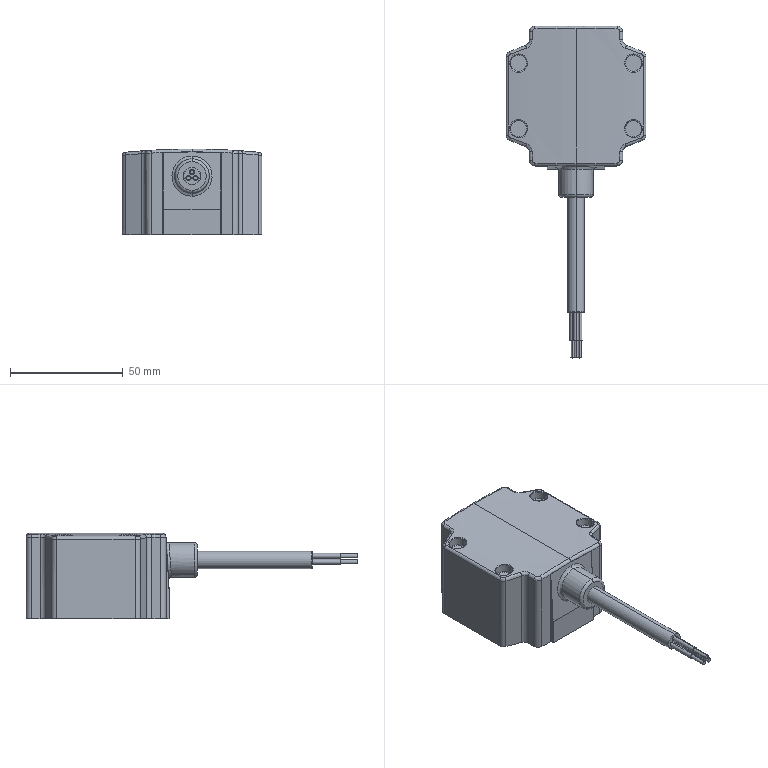Part | STEP file | HF-KE23B_BACK | 1 solid | 130 faces | box 61.976 x 147.066 x 38.075 mm | volume 133952 mm3 | cylinder 51 | spline 34 | plane 30 | torus 15 | commonest cylinder face diameters 5.08 x12 7.62 x10 1.778 x6 2.286 x6 2.54 x6 0.102 x3